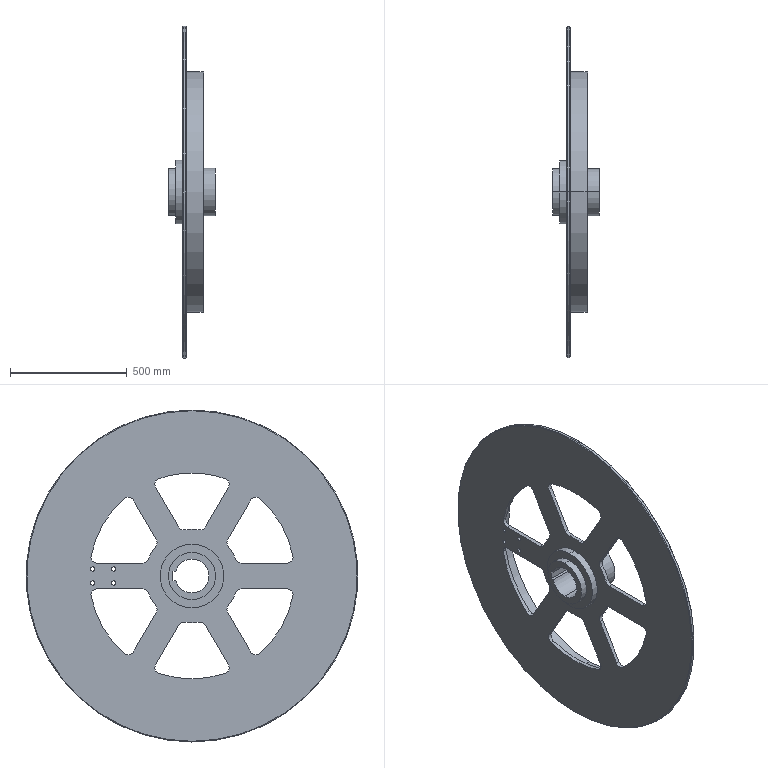Part | SolidWorks | features ICE 5, CirPattern 2, Chamfer 1, Fillet 1, RevCut 1, Revolution 1 | 1 solid | 93 faces | box 201 x 1420 x 1420 mm | volume 29509148 mm3 | cylinder 65 | plane 22 | cone 6 | commonest cylinder face diameters 50 x28 18 x8 400 x7 880 x7 145 x3 202.359 x2